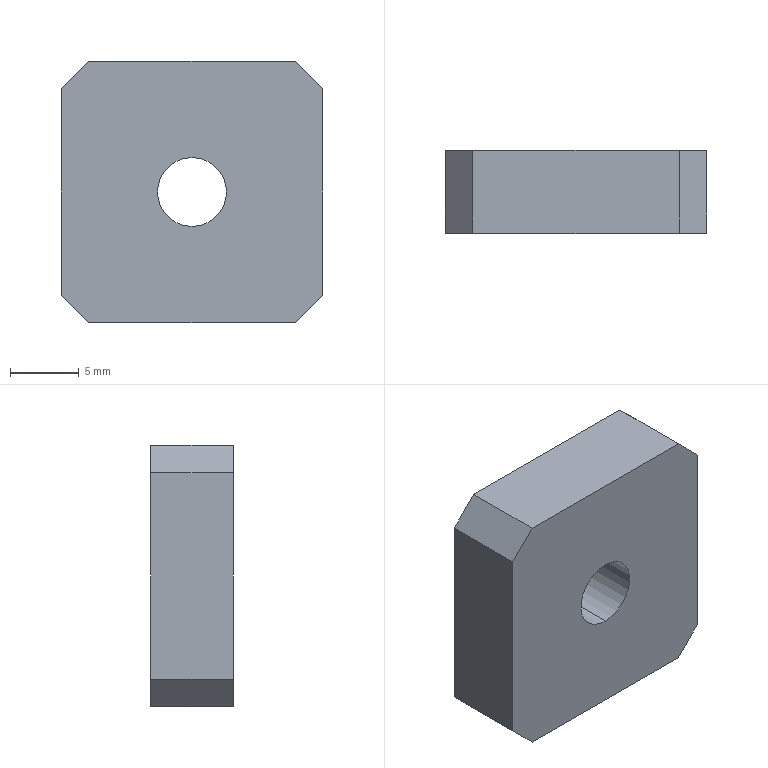Part | NX | features BREP 1 | 1 solid | 12 faces | box 19 x 6 x 19 mm | volume 2000 mm3 | plane 10 | cylinder 2 | commonest cylinder face diameters 5 x2
STEP:
#1=CARTESIAN_POINT('',(9.5,6.,-7.5));
#2=VERTEX_POINT('',#1);
#3=CARTESIAN_POINT('',(7.5,6.,-9.5));
#4=VERTEX_POINT('',#3);
#5=CARTESIAN_POINT('',(7.5,6.,-9.5));
#6=DIRECTION('',(-0.7071,0.,-0.7071));
#7=VECTOR('',#6,1000.);
#8=LINE('',#5,#7);
#9=EDGE_CURVE('',#2,#4,#8,.T.);
#10=ORIENTED_EDGE('',*,*,#9,.F.);
#11=CARTESIAN_POINT('',(9.5,0.,-7.5));
#12=VERTEX_POINT('',#11);
#13=CARTESIAN_POINT('',(9.5,6.,-7.5));
#14=DIRECTION('',(0.,1.,0.));
#15=VECTOR('',#14,1000.);
#16=LINE('',#13,#15);
#17=EDGE_CURVE('',#12,#2,#16,.T.);
#18=ORIENTED_EDGE('',*,*,#17,.F.);
#19=CARTESIAN_POINT('',(7.5,0.,-9.5));
#20=VERTEX_POINT('',#19);
#21=CARTESIAN_POINT('',(8.5,0.,-8.5));
#22=DIRECTION('',(0.7071,0.,0.7071));
#23=VECTOR('',#22,1000.);
#24=LINE('',#21,#23);
#25=EDGE_CURVE('',#20,#12,#24,.T.);
#26=ORIENTED_EDGE('',*,*,#25,.F.);
#27=CARTESIAN_POINT('',(7.5,6.,-9.5));
#28=DIRECTION('',(0.,-1.,0.));
#29=VECTOR('',#28,1000.);
#30=LINE('',#27,#29);
#31=EDGE_CURVE('',#4,#20,#30,.T.);
#32=ORIENTED_EDGE('',*,*,#31,.F.);
#33=EDGE_LOOP('',(#10,#18,#26,#32));
#34=FACE_BOUND('',#33,.T.);
#35=CARTESIAN_POINT('',(7.5,6.,-9.5));
#36=DIRECTION('',(-0.7071,0.,0.7071));
#37=DIRECTION('',(0.,-1.,0.));
#38=AXIS2_PLACEMENT_3D('',#35,#36,#37);
#39=PLANE('',#38);
#40=ADVANCED_FACE('',(#34),#39,.F.);
#41=CARTESIAN_POINT('',(-7.5,6.,-9.5));
#42=VERTEX_POINT('',#41);
#43=CARTESIAN_POINT('',(-9.5,6.,-7.5));
#44=VERTEX_POINT('',#43);
#45=CARTESIAN_POINT('',(-9.5,6.,-7.5));
#46=DIRECTION('',(-0.7071,0.,0.7071));
#47=VECTOR('',#46,1000.);
#48=LINE('',#45,#47);
#49=EDGE_CURVE('',#42,#44,#48,.T.);
#50=ORIENTED_EDGE('',*,*,#49,.F.);
#51=CARTESIAN_POINT('',(-7.5,0.,-9.5));
#52=VERTEX_POINT('',#51);
#53=CARTESIAN_POINT('',(-7.5,6.,-9.5));
#54=DIRECTION('',(0.,1.,0.));
#55=VECTOR('',#54,1000.);
#56=LINE('',#53,#55);
#57=EDGE_CURVE('',#52,#42,#56,.T.);
#58=ORIENTED_EDGE('',*,*,#57,.F.);
#59=CARTESIAN_POINT('',(-9.5,0.,-7.5));
#60=VERTEX_POINT('',#59);
#61=CARTESIAN_POINT('',(-8.5,0.,-8.5));
#62=DIRECTION('',(0.7071,0.,-0.7071));
#63=VECTOR('',#62,1000.);
#64=LINE('',#61,#63);
#65=EDGE_CURVE('',#60,#52,#64,.T.);
#66=ORIENTED_EDGE('',*,*,#65,.F.);
#67=CARTESIAN_POINT('',(-9.5,6.,-7.5));
#68=DIRECTION('',(0.,-1.,0.));
#69=VECTOR('',#68,1000.);
#70=LINE('',#67,#69);
#71=EDGE_CURVE('',#44,#60,#70,.T.);
#72=ORIENTED_EDGE('',*,*,#71,.F.);
#73=EDGE_LOOP('',(#50,#58,#66,#72));
#74=FACE_BOUND('',#73,.T.);
#75=CARTESIAN_POINT('',(-9.5,6.,-7.5));
#76=DIRECTION('',(0.7071,0.,0.7071));
#77=DIRECTION('',(0.,-1.,0.));
#78=AXIS2_PLACEMENT_3D('',#75,#76,#77);
#79=PLANE('',#78);
#80=ADVANCED_FACE('',(#74),#79,.F.);
#81=CARTESIAN_POINT('',(-9.5,6.,7.5));
#82=VERTEX_POINT('',#81);
#83=CARTESIAN_POINT('',(-7.5,6.,9.5));
#84=VERTEX_POINT('',#83);
#85=CARTESIAN_POINT('',(-7.5,6.,9.5));
#86=DIRECTION('',(0.7071,0.,0.7071));
#87=VECTOR('',#86,1000.);
#88=LINE('',#85,#87);
#89=EDGE_CURVE('',#82,#84,#88,.T.);
#90=ORIENTED_EDGE('',*,*,#89,.F.);
#91=CARTESIAN_POINT('',(-9.5,0.,7.5));
#92=VERTEX_POINT('',#91);
#93=CARTESIAN_POINT('',(-9.5,6.,7.5));
#94=DIRECTION('',(0.,1.,0.));
#95=VECTOR('',#94,1000.);
#96=LINE('',#93,#95);
#97=EDGE_CURVE('',#92,#82,#96,.T.);
#98=ORIENTED_EDGE('',*,*,#97,.F.);
#99=CARTESIAN_POINT('',(-7.5,0.,9.5));
#100=VERTEX_POINT('',#99);
#101=CARTESIAN_POINT('',(-8.5,0.,8.5));
#102=DIRECTION('',(-0.7071,0.,-0.7071));
#103=VECTOR('',#102,1000.);
#104=LINE('',#101,#103);
#105=EDGE_CURVE('',#100,#92,#104,.T.);
#106=ORIENTED_EDGE('',*,*,#105,.F.);
#107=CARTESIAN_POINT('',(-7.5,6.,9.5));
#108=DIRECTION('',(0.,-1.,0.));
#109=VECTOR('',#108,1000.);
#110=LINE('',#107,#109);
#111=EDGE_CURVE('',#84,#100,#110,.T.);
#112=ORIENTED_EDGE('',*,*,#111,.F.);
#113=EDGE_LOOP('',(#90,#98,#106,#112));
#114=FACE_BOUND('',#113,.T.);
#115=CARTESIAN_POINT('',(-7.5,6.,9.5));
#116=DIRECTION('',(0.7071,0.,-0.7071));
#117=DIRECTION('',(0.,-1.,0.));
#118=AXIS2_PLACEMENT_3D('',#115,#116,#117);
#119=PLANE('',#118);
#120=ADVANCED_FACE('',(#114),#119,.F.);
#121=CARTESIAN_POINT('',(7.5,6.,9.5));
#122=VERTEX_POINT('',#121);
#123=CARTESIAN_POINT('',(9.5,6.,7.5));
#124=VERTEX_POINT('',#123);
#125=CARTESIAN_POINT('',(9.5,6.,7.5));
#126=DIRECTION('',(0.7071,0.,-0.7071));
#127=VECTOR('',#126,1000.);
#128=LINE('',#125,#127);
#129=EDGE_CURVE('',#122,#124,#128,.T.);
#130=ORIENTED_EDGE('',*,*,#129,.F.);
#131=CARTESIAN_POINT('',(7.5,0.,9.5));
#132=VERTEX_POINT('',#131);
#133=CARTESIAN_POINT('',(7.5,6.,9.5));
#134=DIRECTION('',(0.,1.,0.));
#135=VECTOR('',#134,1000.);
#136=LINE('',#133,#135);
#137=EDGE_CURVE('',#132,#122,#136,.T.);
#138=ORIENTED_EDGE('',*,*,#137,.F.);
#139=CARTESIAN_POINT('',(9.5,0.,7.5));
#140=VERTEX_POINT('',#139);
#141=CARTESIAN_POINT('',(8.5,0.,8.5));
#142=DIRECTION('',(-0.7071,0.,0.7071));
#143=VECTOR('',#142,1000.);
#144=LINE('',#141,#143);
#145=EDGE_CURVE('',#140,#132,#144,.T.);
#146=ORIENTED_EDGE('',*,*,#145,.F.);
#147=CARTESIAN_POINT('',(9.5,6.,7.5));
#148=DIRECTION('',(0.,-1.,0.));
#149=VECTOR('',#148,1000.);
#150=LINE('',#147,#149);
#151=EDGE_CURVE('',#124,#140,#150,.T.);
#152=ORIENTED_EDGE('',*,*,#151,.F.);
#153=EDGE_LOOP('',(#130,#138,#146,#152));
#154=FACE_BOUND('',#153,.T.);
#155=CARTESIAN_POINT('',(9.5,6.,7.5));
#156=DIRECTION('',(-0.7071,0.,-0.7071));
#157=DIRECTION('',(0.,-1.,0.));
#158=AXIS2_PLACEMENT_3D('',#155,#156,#157);
#159=PLANE('',#158);
#160=ADVANCED_FACE('',(#154),#159,.F.);
#161=CARTESIAN_POINT('',(0.,6.,-2.5));
#162=VERTEX_POINT('',#161);
#163=CARTESIAN_POINT('',(0.,0.,-2.5));
#164=VERTEX_POINT('',#163);
#165=CARTESIAN_POINT('',(0.,6.,-2.5));
#166=DIRECTION('',(0.,1.,0.));
#167=VECTOR('',#166,1000.);
#168=LINE('',#165,#167);
#169=EDGE_CURVE('',#162,#164,#168,.F.);
#170=ORIENTED_EDGE('',*,*,#169,.T.);
#171=CARTESIAN_POINT('',(0.,0.,2.5));
#172=VERTEX_POINT('',#171);
#173=CARTESIAN_POINT('',(0.,0.,0.));
#174=DIRECTION('',(0.,1.,0.));
#175=DIRECTION('',(0.,0.,1.));
#176=AXIS2_PLACEMENT_3D('',#173,#174,#175);
#177=CIRCLE('',#176,2.5);
#178=EDGE_CURVE('',#172,#164,#177,.T.);
#179=ORIENTED_EDGE('',*,*,#178,.F.);
#180=CARTESIAN_POINT('',(0.,6.,2.5));
#181=VERTEX_POINT('',#180);
#182=CARTESIAN_POINT('',(0.,6.,2.5));
#183=DIRECTION('',(0.,1.,0.));
#184=VECTOR('',#183,1000.);
#185=LINE('',#182,#184);
#186=EDGE_CURVE('',#181,#172,#185,.F.);
#187=ORIENTED_EDGE('',*,*,#186,.F.);
#188=CARTESIAN_POINT('',(0.,6.,0.));
#189=DIRECTION('',(0.,1.,0.));
#190=DIRECTION('',(0.,0.,1.));
#191=AXIS2_PLACEMENT_3D('',#188,#189,#190);
#192=CIRCLE('',#191,2.5);
#193=EDGE_CURVE('',#181,#162,#192,.T.);
#194=ORIENTED_EDGE('',*,*,#193,.T.);
#195=EDGE_LOOP('',(#170,#179,#187,#194));
#196=FACE_BOUND('',#195,.T.);
#197=CARTESIAN_POINT('',(0.,6.,0.));
#198=DIRECTION('',(0.,1.,0.));
#199=DIRECTION('',(0.,0.,1.));
#200=AXIS2_PLACEMENT_3D('',#197,#198,#199);
#201=CYLINDRICAL_SURFACE('',#200,2.5);
#202=ADVANCED_FACE('',(#196),#201,.F.);
#203=CARTESIAN_POINT('',(9.5,0.,9.5));
#204=DIRECTION('',(0.,0.,-1.));
#205=VECTOR('',#204,1000.);
#206=LINE('',#203,#205);
#207=EDGE_CURVE('',#140,#12,#206,.T.);
#208=ORIENTED_EDGE('',*,*,#207,.F.);
#209=ORIENTED_EDGE('',*,*,#145,.T.);
#210=CARTESIAN_POINT('',(-9.5,0.,9.5));
#211=DIRECTION('',(1.,0.,0.));
#212=VECTOR('',#211,1000.);
#213=LINE('',#210,#212);
#214=EDGE_CURVE('',#100,#132,#213,.T.);
#215=ORIENTED_EDGE('',*,*,#214,.F.);
#216=ORIENTED_EDGE('',*,*,#105,.T.);
#217=CARTESIAN_POINT('',(-9.5,0.,9.5));
#218=DIRECTION('',(0.,0.,1.));
#219=VECTOR('',#218,1000.);
#220=LINE('',#217,#219);
#221=EDGE_CURVE('',#60,#92,#220,.T.);
#222=ORIENTED_EDGE('',*,*,#221,.F.);
#223=ORIENTED_EDGE('',*,*,#65,.T.);
#224=CARTESIAN_POINT('',(-9.5,0.,-9.5));
#225=DIRECTION('',(-1.,0.,0.));
#226=VECTOR('',#225,1000.);
#227=LINE('',#224,#226);
#228=EDGE_CURVE('',#20,#52,#227,.T.);
#229=ORIENTED_EDGE('',*,*,#228,.F.);
#230=ORIENTED_EDGE('',*,*,#25,.T.);
#231=EDGE_LOOP('',(#208,#209,#215,#216,#222,#223,#229,#230));
#232=FACE_BOUND('',#231,.T.);
#233=ORIENTED_EDGE('',*,*,#178,.T.);
#234=CARTESIAN_POINT('',(0.,0.,0.));
#235=DIRECTION('',(0.,1.,0.));
#236=DIRECTION('',(0.,0.,1.));
#237=AXIS2_PLACEMENT_3D('',#234,#235,#236);
#238=CIRCLE('',#237,2.5);
#239=EDGE_CURVE('',#164,#172,#238,.T.);
#240=ORIENTED_EDGE('',*,*,#239,.T.);
#241=EDGE_LOOP('',(#233,#240));
#242=FACE_BOUND('',#241,.T.);
#243=CARTESIAN_POINT('',(0.,0.,0.));
#244=DIRECTION('',(0.,-1.,0.));
#245=DIRECTION('',(0.,0.,-1.));
#246=AXIS2_PLACEMENT_3D('',#243,#244,#245);
#247=PLANE('',#246);
#248=ADVANCED_FACE('',(#232,#242),#247,.T.);
#249=CARTESIAN_POINT('',(-9.5,6.,9.5));
#250=DIRECTION('',(1.,0.,0.));
#251=VECTOR('',#250,1000.);
#252=LINE('',#249,#251);
#253=EDGE_CURVE('',#84,#122,#252,.T.);
#254=ORIENTED_EDGE('',*,*,#253,.T.);
#255=ORIENTED_EDGE('',*,*,#129,.T.);
#256=CARTESIAN_POINT('',(9.5,6.,9.5));
#257=DIRECTION('',(0.,0.,-1.));
#258=VECTOR('',#257,1000.);
#259=LINE('',#256,#258);
#260=EDGE_CURVE('',#124,#2,#259,.T.);
#261=ORIENTED_EDGE('',*,*,#260,.T.);
#262=ORIENTED_EDGE('',*,*,#9,.T.);
#263=CARTESIAN_POINT('',(-9.5,6.,-9.5));
#264=DIRECTION('',(-1.,0.,0.));
#265=VECTOR('',#264,1000.);
#266=LINE('',#263,#265);
#267=EDGE_CURVE('',#4,#42,#266,.T.);
#268=ORIENTED_EDGE('',*,*,#267,.T.);
#269=ORIENTED_EDGE('',*,*,#49,.T.);
#270=CARTESIAN_POINT('',(-9.5,6.,9.5));
#271=DIRECTION('',(0.,0.,1.));
#272=VECTOR('',#271,1000.);
#273=LINE('',#270,#272);
#274=EDGE_CURVE('',#44,#82,#273,.T.);
#275=ORIENTED_EDGE('',*,*,#274,.T.);
#276=ORIENTED_EDGE('',*,*,#89,.T.);
#277=EDGE_LOOP('',(#254,#255,#261,#262,#268,#269,#275,#276));
#278=FACE_BOUND('',#277,.T.);
#279=ORIENTED_EDGE('',*,*,#193,.F.);
#280=CARTESIAN_POINT('',(0.,6.,0.));
#281=DIRECTION('',(0.,1.,0.));
#282=DIRECTION('',(0.,0.,1.));
#283=AXIS2_PLACEMENT_3D('',#280,#281,#282);
#284=CIRCLE('',#283,2.5);
#285=EDGE_CURVE('',#162,#181,#284,.T.);
#286=ORIENTED_EDGE('',*,*,#285,.F.);
#287=EDGE_LOOP('',(#279,#286));
#288=FACE_BOUND('',#287,.T.);
#289=CARTESIAN_POINT('',(0.,6.,0.));
#290=DIRECTION('',(0.,-1.,0.));
#291=DIRECTION('',(0.,0.,-1.));
#292=AXIS2_PLACEMENT_3D('',#289,#290,#291);
#293=PLANE('',#292);
#294=ADVANCED_FACE('',(#278,#288),#293,.F.);
#295=ORIENTED_EDGE('',*,*,#214,.T.);
#296=ORIENTED_EDGE('',*,*,#137,.T.);
#297=ORIENTED_EDGE('',*,*,#253,.F.);
#298=ORIENTED_EDGE('',*,*,#111,.T.);
#299=EDGE_LOOP('',(#295,#296,#297,#298));
#300=FACE_BOUND('',#299,.T.);
#301=CARTESIAN_POINT('',(-9.5,6.,9.5));
#302=DIRECTION('',(0.,0.,-1.));
#303=DIRECTION('',(-1.,0.,0.));
#304=AXIS2_PLACEMENT_3D('',#301,#302,#303);
#305=PLANE('',#304);
#306=ADVANCED_FACE('',(#300),#305,.F.);
#307=ORIENTED_EDGE('',*,*,#221,.T.);
#308=ORIENTED_EDGE('',*,*,#97,.T.);
#309=ORIENTED_EDGE('',*,*,#274,.F.);
#310=ORIENTED_EDGE('',*,*,#71,.T.);
#311=EDGE_LOOP('',(#307,#308,#309,#310));
#312=FACE_BOUND('',#311,.T.);
#313=CARTESIAN_POINT('',(-9.5,6.,9.5));
#314=DIRECTION('',(1.,0.,0.));
#315=DIRECTION('',(0.,0.,-1.));
#316=AXIS2_PLACEMENT_3D('',#313,#314,#315);
#317=PLANE('',#316);
#318=ADVANCED_FACE('',(#312),#317,.F.);
#319=ORIENTED_EDGE('',*,*,#228,.T.);
#320=ORIENTED_EDGE('',*,*,#57,.T.);
#321=ORIENTED_EDGE('',*,*,#267,.F.);
#322=ORIENTED_EDGE('',*,*,#31,.T.);
#323=EDGE_LOOP('',(#319,#320,#321,#322));
#324=FACE_BOUND('',#323,.T.);
#325=CARTESIAN_POINT('',(-9.5,6.,-9.5));
#326=DIRECTION('',(0.,0.,1.));
#327=DIRECTION('',(1.,0.,0.));
#328=AXIS2_PLACEMENT_3D('',#325,#326,#327);
#329=PLANE('',#328);
#330=ADVANCED_FACE('',(#324),#329,.F.);
#331=ORIENTED_EDGE('',*,*,#260,.F.);
#332=ORIENTED_EDGE('',*,*,#151,.T.);
#333=ORIENTED_EDGE('',*,*,#207,.T.);
#334=ORIENTED_EDGE('',*,*,#17,.T.);
#335=EDGE_LOOP('',(#331,#332,#333,#334));
#336=FACE_BOUND('',#335,.T.);
#337=CARTESIAN_POINT('',(9.5,6.,9.5));
#338=DIRECTION('',(-1.,0.,0.));
#339=DIRECTION('',(0.,0.,1.));
#340=AXIS2_PLACEMENT_3D('',#337,#338,#339);
#341=PLANE('',#340);
#342=ADVANCED_FACE('',(#336),#341,.F.);
#343=ORIENTED_EDGE('',*,*,#239,.F.);
#344=ORIENTED_EDGE('',*,*,#169,.F.);
#345=ORIENTED_EDGE('',*,*,#285,.T.);
#346=ORIENTED_EDGE('',*,*,#186,.T.);
#347=EDGE_LOOP('',(#343,#344,#345,#346));
#348=FACE_BOUND('',#347,.T.);
#349=CARTESIAN_POINT('',(0.,6.,0.));
#350=DIRECTION('',(0.,1.,0.));
#351=DIRECTION('',(0.,0.,1.));
#352=AXIS2_PLACEMENT_3D('',#349,#350,#351);
#353=CYLINDRICAL_SURFACE('',#352,2.5);
#354=ADVANCED_FACE('',(#348),#353,.F.);
#355=CLOSED_SHELL('',(#40,#80,#120,#160,#202,#248,#294,#306,#318,#330,#342,#354));
#356=MANIFOLD_SOLID_BREP('',#355);
#357=(LENGTH_UNIT()NAMED_UNIT(*)SI_UNIT(.MILLI.,.METRE.));
#358=UNCERTAINTY_MEASURE_WITH_UNIT(LENGTH_MEASURE(0.00001),#357,'','');
#359=(NAMED_UNIT(*)PLANE_ANGLE_UNIT()SI_UNIT($,.RADIAN.));
#360=(NAMED_UNIT(*)SI_UNIT($,.STERADIAN.)SOLID_ANGLE_UNIT());
#361=(GEOMETRIC_REPRESENTATION_CONTEXT(3)GLOBAL_UNCERTAINTY_ASSIGNED_CONTEXT((#358))GLOBAL_UNIT_ASSIGNED_CONTEXT((#357,#359,#360))REPRESENTATION_CONTEXT('',''));
#362=ADVANCED_BREP_SHAPE_REPRESENTATION('',(#356),#361);